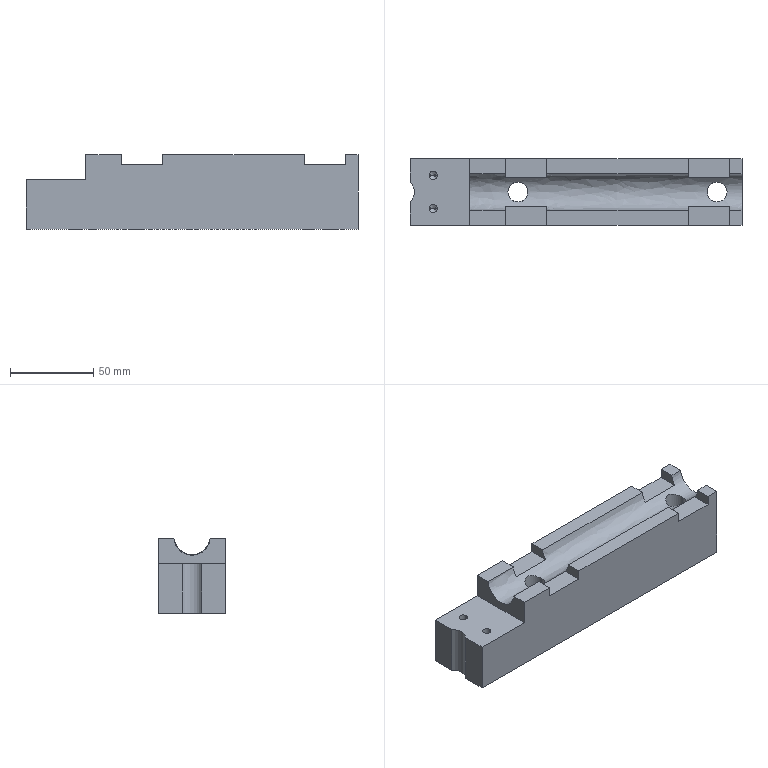CAM job | NX | 3-axis milling, drilling
Tools:
number,name,description,diameter,corner_radius,flute_length,length,flutes
1,D63,Milling Tool-5 Parameters,63.0,0.0,50.0,75.0,2
10,D10,Milling Tool-5 Parameters,10.0,0.0,50.0,75.0,2
6,D6,Milling Tool-5 Parameters,6.0,0.0,50.0,75.0,2
8,R3,Milling Tool-5 Parameters,6.0,3.0,50.0,75.0,2
7,D6A45,Milling Tool-5 Parameters,6.0,0.0,3.0,3.0,2
14,4.8ZT,Drilling Tool,4.8,0.0,35.0,50.0,2
15,5.0JD,Milling Tool-5 Parameters,5.0,0.0,30.0,30.0,4
17,7.0ZT,Drilling Tool,7.0,0.0,35.0,50.0,2
Operations:
program,operation,operation_type,tool,method,geometry_group,spindle_rpm,surface_speed,feed_per_tooth,feed_cut,feed_plunge,cut_length_mm,path_length_mm,cut_time_min,machine_time_min
1,FLOOR_WALL,VolumeBased25DMillingOperation,D63,METHOD,A,6500.0,1286.0,0.0962,1250.0,100.0,1375.0,2701.001,1.1,1.233
1,ADAPTIVE_MILLING,CavityMilling,D10,METHOD,A,9500.0,298.0,0.1579,3000.0,1000.0,11171.706,16650.577,3.75,4.298
1,FLOOR_WALL_1,VolumeBased25DMillingOperation,D6,METHOD,A,9500.0,179.0,0.0658,1250.0,100.0,1567.681,2914.891,1.254,1.389
1,FIXED_CONTOUR,SurfaceContour,D6,METHOD,MCS_MILL,9500.0,179.0,0.1316,2500.0,500.0,15875.639,16093.693,6.42,6.442
1,FIXED_CONTOUR_COPY,SurfaceContour,R3,METHOD,MCS_MILL,9500.0,179.0,0.1842,3500.0,500.0,42608.782,42944.164,12.24,12.273
1,DRILLING_COPY_1,Operation,D6A45,METHOD,A,5000.0,94.0,0.025,250.0,0.0,22.0,328.547,0.088,0.1187
1,DRILLING_COPY_COPY_1,Operation,4.8ZT,METHOD,A,2000.0,15.0,0.03,120.0,0.0,38.884,190.992,0.324,0.3392
1,DRILLING_COPY_COPY_1_COPY,Operation,5.0JD,METHOD,A,1000.0,15.0,0.0125,50.0,0.0,36.0,185.224,0.72,0.7349
1,ZLEVEL_PROFILE_1_COPY_1_COPY,ZLevelMilling,D6A45,METHOD,A,9500.0,179.0,0.0526,1000.0,100.0,631.301,1419.84,0.6313,0.7102
1,ZLEVEL_PROFILE_1_COPY_1_COPY_COPY,ZLevelMilling,D6A45,METHOD,A,9500.0,179.0,0.0526,1000.0,100.0,145.497,473.525,0.1455,0.1783
1,ZLEVEL_PROFILE_1_COPY_1_COPY_COPY_COPY,ZLevelMilling,D6A45,METHOD,A,9500.0,179.0,0.0526,1000.0,100.0,107.19,716.21,0.1072,0.1681
2,FLOOR_WALL_COPY,VolumeBased25DMillingOperation,D63,METHOD,B,6500.0,1286.0,0.0962,1250.0,100.0,1375.0,2701.001,1.1,1.233
2,DRILLING_COPY_1_COPY,Operation,D6A45,METHOD,B,5000.0,94.0,0.025,250.0,0.0,55.0,441.639,0.22,0.2587
2,DRILLING_COPY_COPY_1_COPY_1,Operation,4.8ZT,METHOD,B,2000.0,15.0,0.03,120.0,0.0,32.884,258.803,0.274,0.2966
2,DRILLING_COPY_COPY_1_COPY_COPY,Operation,5.0JD,METHOD,B,1000.0,15.0,0.0125,50.0,0.0,30.0,253.035,0.6,0.6223
2,DRILLING_COPY_COPY_1_COPY_1_1,Operation,7.0ZT,METHOD,B,2000.0,43.0,0.05,200.0,0.0,102.618,495.903,0.5131,0.5524
2,ZLEVEL_PROFILE_1_COPY_1_COPY_COPY_1,ZLevelMilling,D6A45,METHOD,B,9500.0,179.0,0.0526,1000.0,100.0,724.341,2368.856,0.7243,0.8888